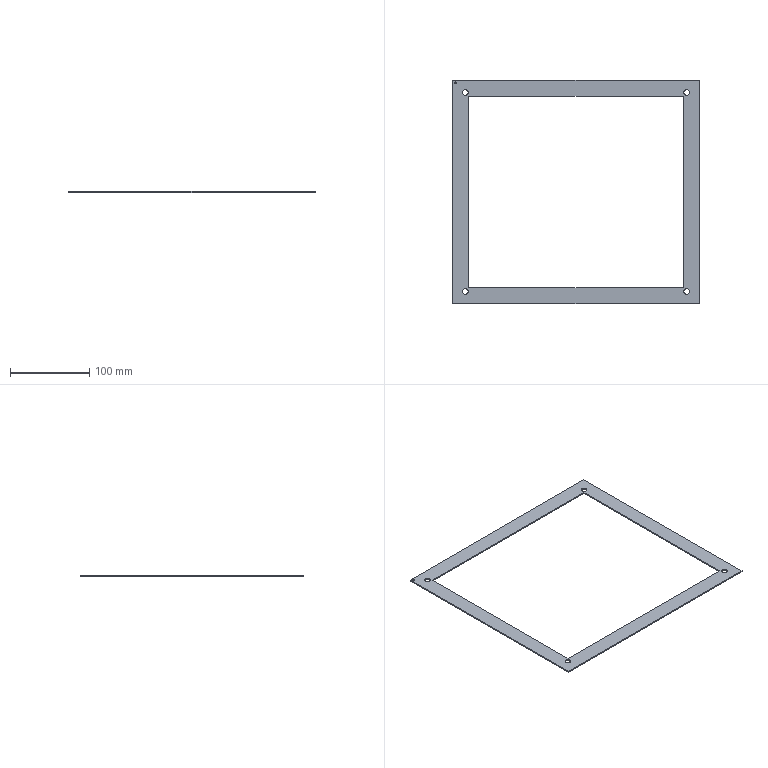Part | SolidWorks | features MirrorStock 1 | 1 solid | 20 faces | box 310 x 281.5 x 1.5 mm | volume 32848 mm3 | cylinder 10 | plane 10 | commonest cylinder face diameters 7.1 x8 2 x2
STEP:
#1=CARTESIAN_POINT('',(2.,278.5,0.));
#2=VERTEX_POINT('',#1);
#3=CARTESIAN_POINT('',(4.,278.5,0.));
#4=VERTEX_POINT('',#3);
#5=CARTESIAN_POINT('',(3.,278.5,0.));
#6=DIRECTION('',(0.,0.,-1.));
#7=DIRECTION('',(-1.,0.,0.));
#8=AXIS2_PLACEMENT_3D('',#5,#6,#7);
#9=CIRCLE('',#8,1.);
#10=EDGE_CURVE('',#2,#4,#9,.T.);
#11=ORIENTED_EDGE('',*,*,#10,.T.);
#12=CARTESIAN_POINT('',(4.,278.5,1.5));
#13=VERTEX_POINT('',#12);
#14=CARTESIAN_POINT('',(4.,278.5,0.));
#15=DIRECTION('',(0.,0.,1.));
#16=VECTOR('',#15,1000.);
#17=LINE('',#14,#16);
#18=EDGE_CURVE('',#4,#13,#17,.T.);
#19=ORIENTED_EDGE('',*,*,#18,.T.);
#20=CARTESIAN_POINT('',(2.,278.5,1.5));
#21=VERTEX_POINT('',#20);
#22=CARTESIAN_POINT('',(3.,278.5,1.5));
#23=DIRECTION('',(0.,0.,-1.));
#24=DIRECTION('',(-1.,0.,0.));
#25=AXIS2_PLACEMENT_3D('',#22,#23,#24);
#26=CIRCLE('',#25,1.);
#27=EDGE_CURVE('',#21,#13,#26,.T.);
#28=ORIENTED_EDGE('',*,*,#27,.F.);
#29=CARTESIAN_POINT('',(2.,278.5,0.));
#30=DIRECTION('',(0.,0.,1.));
#31=VECTOR('',#30,1000.);
#32=LINE('',#29,#31);
#33=EDGE_CURVE('',#2,#21,#32,.T.);
#34=ORIENTED_EDGE('',*,*,#33,.F.);
#35=EDGE_LOOP('',(#11,#19,#28,#34));
#36=FACE_OUTER_BOUND('',#35,.T.);
#37=CARTESIAN_POINT('',(3.,278.5,0.));
#38=DIRECTION('',(0.,0.,1.));
#39=DIRECTION('',(-1.,0.,0.));
#40=AXIS2_PLACEMENT_3D('',#37,#38,#39);
#41=CYLINDRICAL_SURFACE('',#40,1.);
#42=ADVANCED_FACE('',(#36),#41,.F.);
#43=CARTESIAN_POINT('',(19.05,266.,1.5));
#44=VERTEX_POINT('',#43);
#45=CARTESIAN_POINT('',(11.95,266.,1.5));
#46=VERTEX_POINT('',#45);
#47=CARTESIAN_POINT('',(15.5,266.,1.5));
#48=DIRECTION('',(0.,0.,1.));
#49=DIRECTION('',(1.,0.,0.));
#50=AXIS2_PLACEMENT_3D('',#47,#48,#49);
#51=CIRCLE('',#50,3.55);
#52=EDGE_CURVE('',#44,#46,#51,.T.);
#53=ORIENTED_EDGE('',*,*,#52,.T.);
#54=CARTESIAN_POINT('',(11.95,266.,0.));
#55=VERTEX_POINT('',#54);
#56=CARTESIAN_POINT('',(11.95,266.,1.5));
#57=DIRECTION('',(0.,0.,-1.));
#58=VECTOR('',#57,1000.);
#59=LINE('',#56,#58);
#60=EDGE_CURVE('',#46,#55,#59,.T.);
#61=ORIENTED_EDGE('',*,*,#60,.T.);
#62=CARTESIAN_POINT('',(19.05,266.,0.));
#63=VERTEX_POINT('',#62);
#64=CARTESIAN_POINT('',(15.5,266.,0.));
#65=DIRECTION('',(0.,0.,1.));
#66=DIRECTION('',(1.,0.,0.));
#67=AXIS2_PLACEMENT_3D('',#64,#65,#66);
#68=CIRCLE('',#67,3.55);
#69=EDGE_CURVE('',#63,#55,#68,.T.);
#70=ORIENTED_EDGE('',*,*,#69,.F.);
#71=CARTESIAN_POINT('',(19.05,266.,1.5));
#72=DIRECTION('',(0.,0.,-1.));
#73=VECTOR('',#72,1000.);
#74=LINE('',#71,#73);
#75=EDGE_CURVE('',#44,#63,#74,.T.);
#76=ORIENTED_EDGE('',*,*,#75,.F.);
#77=EDGE_LOOP('',(#53,#61,#70,#76));
#78=FACE_OUTER_BOUND('',#77,.T.);
#79=CARTESIAN_POINT('',(15.5,266.,1.5));
#80=DIRECTION('',(0.,0.,-1.));
#81=DIRECTION('',(1.,0.,0.));
#82=AXIS2_PLACEMENT_3D('',#79,#80,#81);
#83=CYLINDRICAL_SURFACE('',#82,3.55);
#84=ADVANCED_FACE('',(#78),#83,.F.);
#85=CARTESIAN_POINT('',(298.05,266.,1.5));
#86=VERTEX_POINT('',#85);
#87=CARTESIAN_POINT('',(290.95,266.,1.5));
#88=VERTEX_POINT('',#87);
#89=CARTESIAN_POINT('',(294.5,266.,1.5));
#90=DIRECTION('',(0.,0.,1.));
#91=DIRECTION('',(1.,0.,0.));
#92=AXIS2_PLACEMENT_3D('',#89,#90,#91);
#93=CIRCLE('',#92,3.55);
#94=EDGE_CURVE('',#86,#88,#93,.T.);
#95=ORIENTED_EDGE('',*,*,#94,.T.);
#96=CARTESIAN_POINT('',(290.95,266.,0.));
#97=VERTEX_POINT('',#96);
#98=CARTESIAN_POINT('',(290.95,266.,1.5));
#99=DIRECTION('',(0.,0.,-1.));
#100=VECTOR('',#99,1000.);
#101=LINE('',#98,#100);
#102=EDGE_CURVE('',#88,#97,#101,.T.);
#103=ORIENTED_EDGE('',*,*,#102,.T.);
#104=CARTESIAN_POINT('',(298.05,266.,0.));
#105=VERTEX_POINT('',#104);
#106=CARTESIAN_POINT('',(294.5,266.,0.));
#107=DIRECTION('',(0.,0.,1.));
#108=DIRECTION('',(1.,0.,0.));
#109=AXIS2_PLACEMENT_3D('',#106,#107,#108);
#110=CIRCLE('',#109,3.55);
#111=EDGE_CURVE('',#105,#97,#110,.T.);
#112=ORIENTED_EDGE('',*,*,#111,.F.);
#113=CARTESIAN_POINT('',(298.05,266.,1.5));
#114=DIRECTION('',(0.,0.,-1.));
#115=VECTOR('',#114,1000.);
#116=LINE('',#113,#115);
#117=EDGE_CURVE('',#86,#105,#116,.T.);
#118=ORIENTED_EDGE('',*,*,#117,.F.);
#119=EDGE_LOOP('',(#95,#103,#112,#118));
#120=FACE_OUTER_BOUND('',#119,.T.);
#121=CARTESIAN_POINT('',(294.5,266.,1.5));
#122=DIRECTION('',(0.,0.,-1.));
#123=DIRECTION('',(1.,0.,0.));
#124=AXIS2_PLACEMENT_3D('',#121,#122,#123);
#125=CYLINDRICAL_SURFACE('',#124,3.55);
#126=ADVANCED_FACE('',(#120),#125,.F.);
#127=CARTESIAN_POINT('',(298.05,15.5,1.5));
#128=VERTEX_POINT('',#127);
#129=CARTESIAN_POINT('',(290.95,15.5,1.5));
#130=VERTEX_POINT('',#129);
#131=CARTESIAN_POINT('',(294.5,15.5,1.5));
#132=DIRECTION('',(0.,0.,1.));
#133=DIRECTION('',(1.,0.,0.));
#134=AXIS2_PLACEMENT_3D('',#131,#132,#133);
#135=CIRCLE('',#134,3.55);
#136=EDGE_CURVE('',#128,#130,#135,.T.);
#137=ORIENTED_EDGE('',*,*,#136,.T.);
#138=CARTESIAN_POINT('',(290.95,15.5,0.));
#139=VERTEX_POINT('',#138);
#140=CARTESIAN_POINT('',(290.95,15.5,1.5));
#141=DIRECTION('',(0.,0.,-1.));
#142=VECTOR('',#141,1000.);
#143=LINE('',#140,#142);
#144=EDGE_CURVE('',#130,#139,#143,.T.);
#145=ORIENTED_EDGE('',*,*,#144,.T.);
#146=CARTESIAN_POINT('',(298.05,15.5,0.));
#147=VERTEX_POINT('',#146);
#148=CARTESIAN_POINT('',(294.5,15.5,0.));
#149=DIRECTION('',(0.,0.,1.));
#150=DIRECTION('',(1.,0.,0.));
#151=AXIS2_PLACEMENT_3D('',#148,#149,#150);
#152=CIRCLE('',#151,3.55);
#153=EDGE_CURVE('',#147,#139,#152,.T.);
#154=ORIENTED_EDGE('',*,*,#153,.F.);
#155=CARTESIAN_POINT('',(298.05,15.5,1.5));
#156=DIRECTION('',(0.,0.,-1.));
#157=VECTOR('',#156,1000.);
#158=LINE('',#155,#157);
#159=EDGE_CURVE('',#128,#147,#158,.T.);
#160=ORIENTED_EDGE('',*,*,#159,.F.);
#161=EDGE_LOOP('',(#137,#145,#154,#160));
#162=FACE_OUTER_BOUND('',#161,.T.);
#163=CARTESIAN_POINT('',(294.5,15.5,1.5));
#164=DIRECTION('',(0.,0.,-1.));
#165=DIRECTION('',(1.,0.,0.));
#166=AXIS2_PLACEMENT_3D('',#163,#164,#165);
#167=CYLINDRICAL_SURFACE('',#166,3.55);
#168=ADVANCED_FACE('',(#162),#167,.F.);
#169=CARTESIAN_POINT('',(19.05,15.5,1.5));
#170=VERTEX_POINT('',#169);
#171=CARTESIAN_POINT('',(11.95,15.5,1.5));
#172=VERTEX_POINT('',#171);
#173=CARTESIAN_POINT('',(15.5,15.5,1.5));
#174=DIRECTION('',(0.,0.,1.));
#175=DIRECTION('',(1.,0.,0.));
#176=AXIS2_PLACEMENT_3D('',#173,#174,#175);
#177=CIRCLE('',#176,3.55);
#178=EDGE_CURVE('',#170,#172,#177,.T.);
#179=ORIENTED_EDGE('',*,*,#178,.T.);
#180=CARTESIAN_POINT('',(11.95,15.5,0.));
#181=VERTEX_POINT('',#180);
#182=CARTESIAN_POINT('',(11.95,15.5,1.5));
#183=DIRECTION('',(0.,0.,-1.));
#184=VECTOR('',#183,1000.);
#185=LINE('',#182,#184);
#186=EDGE_CURVE('',#172,#181,#185,.T.);
#187=ORIENTED_EDGE('',*,*,#186,.T.);
#188=CARTESIAN_POINT('',(19.05,15.5,0.));
#189=VERTEX_POINT('',#188);
#190=CARTESIAN_POINT('',(15.5,15.5,0.));
#191=DIRECTION('',(0.,0.,1.));
#192=DIRECTION('',(1.,0.,0.));
#193=AXIS2_PLACEMENT_3D('',#190,#191,#192);
#194=CIRCLE('',#193,3.55);
#195=EDGE_CURVE('',#189,#181,#194,.T.);
#196=ORIENTED_EDGE('',*,*,#195,.F.);
#197=CARTESIAN_POINT('',(19.05,15.5,1.5));
#198=DIRECTION('',(0.,0.,-1.));
#199=VECTOR('',#198,1000.);
#200=LINE('',#197,#199);
#201=EDGE_CURVE('',#170,#189,#200,.T.);
#202=ORIENTED_EDGE('',*,*,#201,.F.);
#203=EDGE_LOOP('',(#179,#187,#196,#202));
#204=FACE_OUTER_BOUND('',#203,.T.);
#205=CARTESIAN_POINT('',(15.5,15.5,1.5));
#206=DIRECTION('',(0.,0.,-1.));
#207=DIRECTION('',(1.,0.,0.));
#208=AXIS2_PLACEMENT_3D('',#205,#206,#207);
#209=CYLINDRICAL_SURFACE('',#208,3.55);
#210=ADVANCED_FACE('',(#204),#209,.F.);
#211=CARTESIAN_POINT('',(0.,281.5,0.));
#212=VERTEX_POINT('',#211);
#213=CARTESIAN_POINT('',(0.,0.,0.));
#214=VERTEX_POINT('',#213);
#215=CARTESIAN_POINT('',(0.,0.,0.));
#216=DIRECTION('',(0.,-1.,0.));
#217=VECTOR('',#216,1000.);
#218=LINE('',#215,#217);
#219=EDGE_CURVE('',#212,#214,#218,.T.);
#220=ORIENTED_EDGE('',*,*,#219,.T.);
#221=CARTESIAN_POINT('',(0.,0.,1.5));
#222=VERTEX_POINT('',#221);
#223=CARTESIAN_POINT('',(0.,0.,1.5));
#224=DIRECTION('',(0.,0.,-1.));
#225=VECTOR('',#224,1000.);
#226=LINE('',#223,#225);
#227=EDGE_CURVE('',#222,#214,#226,.T.);
#228=ORIENTED_EDGE('',*,*,#227,.F.);
#229=CARTESIAN_POINT('',(0.,281.5,1.5));
#230=VERTEX_POINT('',#229);
#231=CARTESIAN_POINT('',(0.,0.,1.5));
#232=DIRECTION('',(0.,-1.,0.));
#233=VECTOR('',#232,1000.);
#234=LINE('',#231,#233);
#235=EDGE_CURVE('',#230,#222,#234,.T.);
#236=ORIENTED_EDGE('',*,*,#235,.F.);
#237=CARTESIAN_POINT('',(0.,281.5,1.5));
#238=DIRECTION('',(0.,0.,-1.));
#239=VECTOR('',#238,1000.);
#240=LINE('',#237,#239);
#241=EDGE_CURVE('',#230,#212,#240,.T.);
#242=ORIENTED_EDGE('',*,*,#241,.T.);
#243=EDGE_LOOP('',(#220,#228,#236,#242));
#244=FACE_OUTER_BOUND('',#243,.T.);
#245=CARTESIAN_POINT('',(0.,0.,1.5));
#246=DIRECTION('',(-1.,0.,0.));
#247=DIRECTION('',(0.,0.,-1.));
#248=AXIS2_PLACEMENT_3D('',#245,#246,#247);
#249=PLANE('',#248);
#250=ADVANCED_FACE('',(#244),#249,.T.);
#251=CARTESIAN_POINT('',(310.,281.5,0.));
#252=VERTEX_POINT('',#251);
#253=CARTESIAN_POINT('',(0.,281.5,0.));
#254=DIRECTION('',(-1.,0.,0.));
#255=VECTOR('',#254,1000.);
#256=LINE('',#253,#255);
#257=EDGE_CURVE('',#252,#212,#256,.T.);
#258=ORIENTED_EDGE('',*,*,#257,.T.);
#259=ORIENTED_EDGE('',*,*,#241,.F.);
#260=CARTESIAN_POINT('',(310.,281.5,1.5));
#261=VERTEX_POINT('',#260);
#262=CARTESIAN_POINT('',(0.,281.5,1.5));
#263=DIRECTION('',(-1.,0.,0.));
#264=VECTOR('',#263,1000.);
#265=LINE('',#262,#264);
#266=EDGE_CURVE('',#261,#230,#265,.T.);
#267=ORIENTED_EDGE('',*,*,#266,.F.);
#268=CARTESIAN_POINT('',(310.,281.5,1.5));
#269=DIRECTION('',(0.,0.,-1.));
#270=VECTOR('',#269,1000.);
#271=LINE('',#268,#270);
#272=EDGE_CURVE('',#261,#252,#271,.T.);
#273=ORIENTED_EDGE('',*,*,#272,.T.);
#274=EDGE_LOOP('',(#258,#259,#267,#273));
#275=FACE_OUTER_BOUND('',#274,.T.);
#276=CARTESIAN_POINT('',(0.,281.5,1.5));
#277=DIRECTION('',(0.,1.,0.));
#278=DIRECTION('',(0.,0.,-1.));
#279=AXIS2_PLACEMENT_3D('',#276,#277,#278);
#280=PLANE('',#279);
#281=ADVANCED_FACE('',(#275),#280,.T.);
#282=CARTESIAN_POINT('',(310.,0.,0.));
#283=VERTEX_POINT('',#282);
#284=CARTESIAN_POINT('',(310.,0.,0.));
#285=DIRECTION('',(0.,1.,0.));
#286=VECTOR('',#285,1000.);
#287=LINE('',#284,#286);
#288=EDGE_CURVE('',#283,#252,#287,.T.);
#289=ORIENTED_EDGE('',*,*,#288,.T.);
#290=ORIENTED_EDGE('',*,*,#272,.F.);
#291=CARTESIAN_POINT('',(310.,0.,1.5));
#292=VERTEX_POINT('',#291);
#293=CARTESIAN_POINT('',(310.,0.,1.5));
#294=DIRECTION('',(0.,1.,0.));
#295=VECTOR('',#294,1000.);
#296=LINE('',#293,#295);
#297=EDGE_CURVE('',#292,#261,#296,.T.);
#298=ORIENTED_EDGE('',*,*,#297,.F.);
#299=CARTESIAN_POINT('',(310.,0.,1.5));
#300=DIRECTION('',(0.,0.,-1.));
#301=VECTOR('',#300,1000.);
#302=LINE('',#299,#301);
#303=EDGE_CURVE('',#292,#283,#302,.T.);
#304=ORIENTED_EDGE('',*,*,#303,.T.);
#305=EDGE_LOOP('',(#289,#290,#298,#304));
#306=FACE_OUTER_BOUND('',#305,.T.);
#307=CARTESIAN_POINT('',(310.,0.,1.5));
#308=DIRECTION('',(1.,0.,0.));
#309=DIRECTION('',(0.,0.,1.));
#310=AXIS2_PLACEMENT_3D('',#307,#308,#309);
#311=PLANE('',#310);
#312=ADVANCED_FACE('',(#306),#311,.T.);
#313=CARTESIAN_POINT('',(0.,0.,0.));
#314=DIRECTION('',(1.,0.,0.));
#315=VECTOR('',#314,1000.);
#316=LINE('',#313,#315);
#317=EDGE_CURVE('',#214,#283,#316,.T.);
#318=ORIENTED_EDGE('',*,*,#317,.T.);
#319=ORIENTED_EDGE('',*,*,#303,.F.);
#320=CARTESIAN_POINT('',(0.,0.,1.5));
#321=DIRECTION('',(1.,0.,0.));
#322=VECTOR('',#321,1000.);
#323=LINE('',#320,#322);
#324=EDGE_CURVE('',#222,#292,#323,.T.);
#325=ORIENTED_EDGE('',*,*,#324,.F.);
#326=ORIENTED_EDGE('',*,*,#227,.T.);
#327=EDGE_LOOP('',(#318,#319,#325,#326));
#328=FACE_OUTER_BOUND('',#327,.T.);
#329=CARTESIAN_POINT('',(0.,0.,1.5));
#330=DIRECTION('',(0.,-1.,0.));
#331=DIRECTION('',(0.,0.,1.));
#332=AXIS2_PLACEMENT_3D('',#329,#330,#331);
#333=PLANE('',#332);
#334=ADVANCED_FACE('',(#328),#333,.T.);
#335=ORIENTED_EDGE('',*,*,#27,.T.);
#336=CARTESIAN_POINT('',(3.,278.5,1.5));
#337=DIRECTION('',(0.,0.,-1.));
#338=DIRECTION('',(-1.,0.,0.));
#339=AXIS2_PLACEMENT_3D('',#336,#337,#338);
#340=CIRCLE('',#339,1.);
#341=EDGE_CURVE('',#13,#21,#340,.T.);
#342=ORIENTED_EDGE('',*,*,#341,.T.);
#343=EDGE_LOOP('',(#335,#342));
#344=FACE_BOUND('',#343,.T.);
#345=ORIENTED_EDGE('',*,*,#52,.F.);
#346=CARTESIAN_POINT('',(15.5,266.,1.5));
#347=DIRECTION('',(0.,0.,1.));
#348=DIRECTION('',(1.,0.,0.));
#349=AXIS2_PLACEMENT_3D('',#346,#347,#348);
#350=CIRCLE('',#349,3.55);
#351=EDGE_CURVE('',#46,#44,#350,.T.);
#352=ORIENTED_EDGE('',*,*,#351,.F.);
#353=EDGE_LOOP('',(#345,#352));
#354=FACE_BOUND('',#353,.T.);
#355=ORIENTED_EDGE('',*,*,#94,.F.);
#356=CARTESIAN_POINT('',(294.5,266.,1.5));
#357=DIRECTION('',(0.,0.,1.));
#358=DIRECTION('',(1.,0.,0.));
#359=AXIS2_PLACEMENT_3D('',#356,#357,#358);
#360=CIRCLE('',#359,3.55);
#361=EDGE_CURVE('',#88,#86,#360,.T.);
#362=ORIENTED_EDGE('',*,*,#361,.F.);
#363=EDGE_LOOP('',(#355,#362));
#364=FACE_BOUND('',#363,.T.);
#365=ORIENTED_EDGE('',*,*,#136,.F.);
#366=CARTESIAN_POINT('',(294.5,15.5,1.5));
#367=DIRECTION('',(0.,0.,1.));
#368=DIRECTION('',(1.,0.,0.));
#369=AXIS2_PLACEMENT_3D('',#366,#367,#368);
#370=CIRCLE('',#369,3.55);
#371=EDGE_CURVE('',#130,#128,#370,.T.);
#372=ORIENTED_EDGE('',*,*,#371,.F.);
#373=EDGE_LOOP('',(#365,#372));
#374=FACE_BOUND('',#373,.T.);
#375=ORIENTED_EDGE('',*,*,#178,.F.);
#376=CARTESIAN_POINT('',(15.5,15.5,1.5));
#377=DIRECTION('',(0.,0.,1.));
#378=DIRECTION('',(1.,0.,0.));
#379=AXIS2_PLACEMENT_3D('',#376,#377,#378);
#380=CIRCLE('',#379,3.55);
#381=EDGE_CURVE('',#172,#170,#380,.T.);
#382=ORIENTED_EDGE('',*,*,#381,.F.);
#383=EDGE_LOOP('',(#375,#382));
#384=FACE_BOUND('',#383,.T.);
#385=CARTESIAN_POINT('',(20.,20.,1.5));
#386=VERTEX_POINT('',#385);
#387=CARTESIAN_POINT('',(290.,20.,1.5));
#388=VERTEX_POINT('',#387);
#389=CARTESIAN_POINT('',(20.,20.,1.5));
#390=DIRECTION('',(1.,0.,0.));
#391=VECTOR('',#390,1000.);
#392=LINE('',#389,#391);
#393=EDGE_CURVE('',#386,#388,#392,.T.);
#394=ORIENTED_EDGE('',*,*,#393,.F.);
#395=CARTESIAN_POINT('',(20.,261.5,1.5));
#396=VERTEX_POINT('',#395);
#397=CARTESIAN_POINT('',(20.,20.,1.5));
#398=DIRECTION('',(0.,-1.,0.));
#399=VECTOR('',#398,1000.);
#400=LINE('',#397,#399);
#401=EDGE_CURVE('',#396,#386,#400,.T.);
#402=ORIENTED_EDGE('',*,*,#401,.F.);
#403=CARTESIAN_POINT('',(290.,261.5,1.5));
#404=VERTEX_POINT('',#403);
#405=CARTESIAN_POINT('',(20.,261.5,1.5));
#406=DIRECTION('',(-1.,0.,0.));
#407=VECTOR('',#406,1000.);
#408=LINE('',#405,#407);
#409=EDGE_CURVE('',#404,#396,#408,.T.);
#410=ORIENTED_EDGE('',*,*,#409,.F.);
#411=CARTESIAN_POINT('',(290.,20.,1.5));
#412=DIRECTION('',(0.,1.,0.));
#413=VECTOR('',#412,1000.);
#414=LINE('',#411,#413);
#415=EDGE_CURVE('',#388,#404,#414,.T.);
#416=ORIENTED_EDGE('',*,*,#415,.F.);
#417=EDGE_LOOP('',(#394,#402,#410,#416));
#418=FACE_BOUND('',#417,.T.);
#419=ORIENTED_EDGE('',*,*,#235,.T.);
#420=ORIENTED_EDGE('',*,*,#324,.T.);
#421=ORIENTED_EDGE('',*,*,#297,.T.);
#422=ORIENTED_EDGE('',*,*,#266,.T.);
#423=EDGE_LOOP('',(#419,#420,#421,#422));
#424=FACE_OUTER_BOUND('',#423,.T.);
#425=CARTESIAN_POINT('',(0.,0.,1.5));
#426=DIRECTION('',(0.,0.,1.));
#427=DIRECTION('',(-1.,0.,0.));
#428=AXIS2_PLACEMENT_3D('',#425,#426,#427);
#429=PLANE('',#428);
#430=ADVANCED_FACE('',(#344,#354,#364,#374,#384,#418,#424),#429,.T.);
#431=ORIENTED_EDGE('',*,*,#10,.F.);
#432=CARTESIAN_POINT('',(3.,278.5,0.));
#433=DIRECTION('',(0.,0.,-1.));
#434=DIRECTION('',(-1.,0.,0.));
#435=AXIS2_PLACEMENT_3D('',#432,#433,#434);
#436=CIRCLE('',#435,1.);
#437=EDGE_CURVE('',#4,#2,#436,.T.);
#438=ORIENTED_EDGE('',*,*,#437,.F.);
#439=EDGE_LOOP('',(#431,#438));
#440=FACE_BOUND('',#439,.T.);
#441=ORIENTED_EDGE('',*,*,#69,.T.);
#442=CARTESIAN_POINT('',(15.5,266.,0.));
#443=DIRECTION('',(0.,0.,1.));
#444=DIRECTION('',(1.,0.,0.));
#445=AXIS2_PLACEMENT_3D('',#442,#443,#444);
#446=CIRCLE('',#445,3.55);
#447=EDGE_CURVE('',#55,#63,#446,.T.);
#448=ORIENTED_EDGE('',*,*,#447,.T.);
#449=EDGE_LOOP('',(#441,#448));
#450=FACE_BOUND('',#449,.T.);
#451=ORIENTED_EDGE('',*,*,#111,.T.);
#452=CARTESIAN_POINT('',(294.5,266.,0.));
#453=DIRECTION('',(0.,0.,1.));
#454=DIRECTION('',(1.,0.,0.));
#455=AXIS2_PLACEMENT_3D('',#452,#453,#454);
#456=CIRCLE('',#455,3.55);
#457=EDGE_CURVE('',#97,#105,#456,.T.);
#458=ORIENTED_EDGE('',*,*,#457,.T.);
#459=EDGE_LOOP('',(#451,#458));
#460=FACE_BOUND('',#459,.T.);
#461=ORIENTED_EDGE('',*,*,#153,.T.);
#462=CARTESIAN_POINT('',(294.5,15.5,0.));
#463=DIRECTION('',(0.,0.,1.));
#464=DIRECTION('',(1.,0.,0.));
#465=AXIS2_PLACEMENT_3D('',#462,#463,#464);
#466=CIRCLE('',#465,3.55);
#467=EDGE_CURVE('',#139,#147,#466,.T.);
#468=ORIENTED_EDGE('',*,*,#467,.T.);
#469=EDGE_LOOP('',(#461,#468));
#470=FACE_BOUND('',#469,.T.);
#471=ORIENTED_EDGE('',*,*,#195,.T.);
#472=CARTESIAN_POINT('',(15.5,15.5,0.));
#473=DIRECTION('',(0.,0.,1.));
#474=DIRECTION('',(1.,0.,0.));
#475=AXIS2_PLACEMENT_3D('',#472,#473,#474);
#476=CIRCLE('',#475,3.55);
#477=EDGE_CURVE('',#181,#189,#476,.T.);
#478=ORIENTED_EDGE('',*,*,#477,.T.);
#479=EDGE_LOOP('',(#471,#478));
#480=FACE_BOUND('',#479,.T.);
#481=CARTESIAN_POINT('',(290.,20.,0.));
#482=VERTEX_POINT('',#481);
#483=CARTESIAN_POINT('',(290.,261.5,0.));
#484=VERTEX_POINT('',#483);
#485=CARTESIAN_POINT('',(290.,20.,0.));
#486=DIRECTION('',(0.,1.,0.));
#487=VECTOR('',#486,1000.);
#488=LINE('',#485,#487);
#489=EDGE_CURVE('',#482,#484,#488,.T.);
#490=ORIENTED_EDGE('',*,*,#489,.T.);
#491=CARTESIAN_POINT('',(20.,261.5,0.));
#492=VERTEX_POINT('',#491);
#493=CARTESIAN_POINT('',(20.,261.5,0.));
#494=DIRECTION('',(-1.,0.,0.));
#495=VECTOR('',#494,1000.);
#496=LINE('',#493,#495);
#497=EDGE_CURVE('',#484,#492,#496,.T.);
#498=ORIENTED_EDGE('',*,*,#497,.T.);
#499=CARTESIAN_POINT('',(20.,20.,0.));
#500=VERTEX_POINT('',#499);
#501=CARTESIAN_POINT('',(20.,20.,0.));
#502=DIRECTION('',(0.,-1.,0.));
#503=VECTOR('',#502,1000.);
#504=LINE('',#501,#503);
#505=EDGE_CURVE('',#492,#500,#504,.T.);
#506=ORIENTED_EDGE('',*,*,#505,.T.);
#507=CARTESIAN_POINT('',(20.,20.,0.));
#508=DIRECTION('',(1.,0.,0.));
#509=VECTOR('',#508,1000.);
#510=LINE('',#507,#509);
#511=EDGE_CURVE('',#500,#482,#510,.T.);
#512=ORIENTED_EDGE('',*,*,#511,.T.);
#513=EDGE_LOOP('',(#490,#498,#506,#512));
#514=FACE_BOUND('',#513,.T.);
#515=ORIENTED_EDGE('',*,*,#219,.F.);
#516=ORIENTED_EDGE('',*,*,#257,.F.);
#517=ORIENTED_EDGE('',*,*,#288,.F.);
#518=ORIENTED_EDGE('',*,*,#317,.F.);
#519=EDGE_LOOP('',(#515,#516,#517,#518));
#520=FACE_OUTER_BOUND('',#519,.T.);
#521=CARTESIAN_POINT('',(0.,0.,0.));
#522=DIRECTION('',(0.,0.,1.));
#523=DIRECTION('',(-1.,0.,0.));
#524=AXIS2_PLACEMENT_3D('',#521,#522,#523);
#525=PLANE('',#524);
#526=ADVANCED_FACE('',(#440,#450,#460,#470,#480,#514,#520),#525,.F.);
#527=ORIENTED_EDGE('',*,*,#511,.F.);
#528=CARTESIAN_POINT('',(20.,20.,1.5));
#529=DIRECTION('',(0.,0.,-1.));
#530=VECTOR('',#529,1000.);
#531=LINE('',#528,#530);
#532=EDGE_CURVE('',#386,#500,#531,.T.);
#533=ORIENTED_EDGE('',*,*,#532,.F.);
#534=ORIENTED_EDGE('',*,*,#393,.T.);
#535=CARTESIAN_POINT('',(290.,20.,1.5));
#536=DIRECTION('',(0.,0.,-1.));
#537=VECTOR('',#536,1000.);
#538=LINE('',#535,#537);
#539=EDGE_CURVE('',#388,#482,#538,.T.);
#540=ORIENTED_EDGE('',*,*,#539,.T.);
#541=EDGE_LOOP('',(#527,#533,#534,#540));
#542=FACE_OUTER_BOUND('',#541,.T.);
#543=CARTESIAN_POINT('',(20.,20.,1.5));
#544=DIRECTION('',(0.,-1.,0.));
#545=DIRECTION('',(0.,0.,1.));
#546=AXIS2_PLACEMENT_3D('',#543,#544,#545);
#547=PLANE('',#546);
#548=ADVANCED_FACE('',(#542),#547,.F.);
#549=ORIENTED_EDGE('',*,*,#505,.F.);
#550=CARTESIAN_POINT('',(20.,261.5,1.5));
#551=DIRECTION('',(0.,0.,-1.));
#552=VECTOR('',#551,1000.);
#553=LINE('',#550,#552);
#554=EDGE_CURVE('',#396,#492,#553,.T.);
#555=ORIENTED_EDGE('',*,*,#554,.F.);
#556=ORIENTED_EDGE('',*,*,#401,.T.);
#557=ORIENTED_EDGE('',*,*,#532,.T.);
#558=EDGE_LOOP('',(#549,#555,#556,#557));
#559=FACE_OUTER_BOUND('',#558,.T.);
#560=CARTESIAN_POINT('',(20.,20.,1.5));
#561=DIRECTION('',(-1.,0.,0.));
#562=DIRECTION('',(0.,0.,-1.));
#563=AXIS2_PLACEMENT_3D('',#560,#561,#562);
#564=PLANE('',#563);
#565=ADVANCED_FACE('',(#559),#564,.F.);
#566=ORIENTED_EDGE('',*,*,#497,.F.);
#567=CARTESIAN_POINT('',(290.,261.5,1.5));
#568=DIRECTION('',(0.,0.,-1.));
#569=VECTOR('',#568,1000.);
#570=LINE('',#567,#569);
#571=EDGE_CURVE('',#404,#484,#570,.T.);
#572=ORIENTED_EDGE('',*,*,#571,.F.);
#573=ORIENTED_EDGE('',*,*,#409,.T.);
#574=ORIENTED_EDGE('',*,*,#554,.T.);
#575=EDGE_LOOP('',(#566,#572,#573,#574));
#576=FACE_OUTER_BOUND('',#575,.T.);
#577=CARTESIAN_POINT('',(20.,261.5,1.5));
#578=DIRECTION('',(0.,1.,0.));
#579=DIRECTION('',(0.,0.,-1.));
#580=AXIS2_PLACEMENT_3D('',#577,#578,#579);
#581=PLANE('',#580);
#582=ADVANCED_FACE('',(#576),#581,.F.);
#583=ORIENTED_EDGE('',*,*,#489,.F.);
#584=ORIENTED_EDGE('',*,*,#539,.F.);
#585=ORIENTED_EDGE('',*,*,#415,.T.);
#586=ORIENTED_EDGE('',*,*,#571,.T.);
#587=EDGE_LOOP('',(#583,#584,#585,#586));
#588=FACE_OUTER_BOUND('',#587,.T.);
#589=CARTESIAN_POINT('',(290.,20.,1.5));
#590=DIRECTION('',(1.,0.,0.));
#591=DIRECTION('',(0.,0.,1.));
#592=AXIS2_PLACEMENT_3D('',#589,#590,#591);
#593=PLANE('',#592);
#594=ADVANCED_FACE('',(#588),#593,.F.);
#595=ORIENTED_EDGE('',*,*,#186,.F.);
#596=ORIENTED_EDGE('',*,*,#381,.T.);
#597=ORIENTED_EDGE('',*,*,#201,.T.);
#598=ORIENTED_EDGE('',*,*,#477,.F.);
#599=EDGE_LOOP('',(#595,#596,#597,#598));
#600=FACE_OUTER_BOUND('',#599,.T.);
#601=CARTESIAN_POINT('',(15.5,15.5,1.5));
#602=DIRECTION('',(0.,0.,-1.));
#603=DIRECTION('',(1.,0.,0.));
#604=AXIS2_PLACEMENT_3D('',#601,#602,#603);
#605=CYLINDRICAL_SURFACE('',#604,3.55);
#606=ADVANCED_FACE('',(#600),#605,.F.);
#607=ORIENTED_EDGE('',*,*,#144,.F.);
#608=ORIENTED_EDGE('',*,*,#371,.T.);
#609=ORIENTED_EDGE('',*,*,#159,.T.);
#610=ORIENTED_EDGE('',*,*,#467,.F.);
#611=EDGE_LOOP('',(#607,#608,#609,#610));
#612=FACE_OUTER_BOUND('',#611,.T.);
#613=CARTESIAN_POINT('',(294.5,15.5,1.5));
#614=DIRECTION('',(0.,0.,-1.));
#615=DIRECTION('',(1.,0.,0.));
#616=AXIS2_PLACEMENT_3D('',#613,#614,#615);
#617=CYLINDRICAL_SURFACE('',#616,3.55);
#618=ADVANCED_FACE('',(#612),#617,.F.);
#619=ORIENTED_EDGE('',*,*,#102,.F.);
#620=ORIENTED_EDGE('',*,*,#361,.T.);
#621=ORIENTED_EDGE('',*,*,#117,.T.);
#622=ORIENTED_EDGE('',*,*,#457,.F.);
#623=EDGE_LOOP('',(#619,#620,#621,#622));
#624=FACE_OUTER_BOUND('',#623,.T.);
#625=CARTESIAN_POINT('',(294.5,266.,1.5));
#626=DIRECTION('',(0.,0.,-1.));
#627=DIRECTION('',(1.,0.,0.));
#628=AXIS2_PLACEMENT_3D('',#625,#626,#627);
#629=CYLINDRICAL_SURFACE('',#628,3.55);
#630=ADVANCED_FACE('',(#624),#629,.F.);
#631=ORIENTED_EDGE('',*,*,#60,.F.);
#632=ORIENTED_EDGE('',*,*,#351,.T.);
#633=ORIENTED_EDGE('',*,*,#75,.T.);
#634=ORIENTED_EDGE('',*,*,#447,.F.);
#635=EDGE_LOOP('',(#631,#632,#633,#634));
#636=FACE_OUTER_BOUND('',#635,.T.);
#637=CARTESIAN_POINT('',(15.5,266.,1.5));
#638=DIRECTION('',(0.,0.,-1.));
#639=DIRECTION('',(1.,0.,0.));
#640=AXIS2_PLACEMENT_3D('',#637,#638,#639);
#641=CYLINDRICAL_SURFACE('',#640,3.55);
#642=ADVANCED_FACE('',(#636),#641,.F.);
#643=ORIENTED_EDGE('',*,*,#18,.F.);
#644=ORIENTED_EDGE('',*,*,#437,.T.);
#645=ORIENTED_EDGE('',*,*,#33,.T.);
#646=ORIENTED_EDGE('',*,*,#341,.F.);
#647=EDGE_LOOP('',(#643,#644,#645,#646));
#648=FACE_OUTER_BOUND('',#647,.T.);
#649=CARTESIAN_POINT('',(3.,278.5,0.));
#650=DIRECTION('',(0.,0.,1.));
#651=DIRECTION('',(-1.,0.,0.));
#652=AXIS2_PLACEMENT_3D('',#649,#650,#651);
#653=CYLINDRICAL_SURFACE('',#652,1.);
#654=ADVANCED_FACE('',(#648),#653,.F.);
#655=CLOSED_SHELL('',(#42,#84,#126,#168,#210,#250,#281,#312,#334,#430,#526,#548,#565,#582,#594,#606,#618,#630,#642,#654));
#656=MANIFOLD_SOLID_BREP('',#655);
#657=CARTESIAN_POINT('',(0.,0.,0.));
#658=DIRECTION('',(0.,0.,1.));
#659=DIRECTION('',(1.,0.,0.));
#660=AXIS2_PLACEMENT_3D('',#657,#658,#659);
#661=(LENGTH_UNIT()NAMED_UNIT(*)SI_UNIT(.MILLI.,.METRE.));
#662=UNCERTAINTY_MEASURE_WITH_UNIT(LENGTH_MEASURE(0.00001),#661,'','');
#663=(NAMED_UNIT(*)PLANE_ANGLE_UNIT()SI_UNIT($,.RADIAN.));
#664=(NAMED_UNIT(*)SI_UNIT($,.STERADIAN.)SOLID_ANGLE_UNIT());
#665=(GEOMETRIC_REPRESENTATION_CONTEXT(3)GLOBAL_UNCERTAINTY_ASSIGNED_CONTEXT((#662))GLOBAL_UNIT_ASSIGNED_CONTEXT((#661,#663,#664))REPRESENTATION_CONTEXT('',''));
#666=ADVANCED_BREP_SHAPE_REPRESENTATION('',(#656,#660),#665);